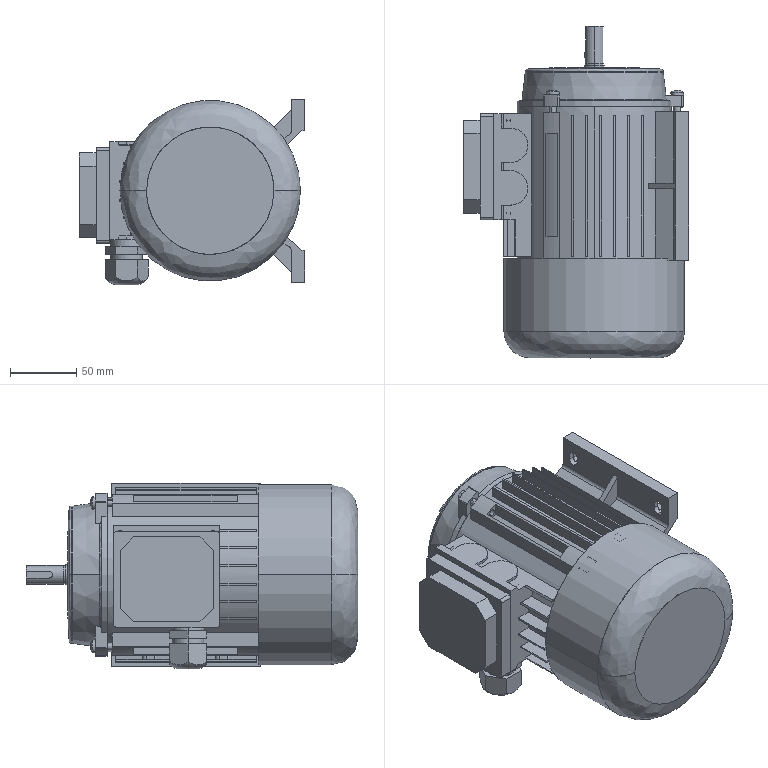Part | SolidWorks | 36 solids | 1239 faces | box 169.5 x 250 x 139.906 mm | volume 665833 mm3 | plane 641 | cylinder 365 | spline 130 | cone 101 | torus 2 | commonest cylinder face diameters 2 x36 3.3 x20 5 x20 132 x19 64 x18 104 x17